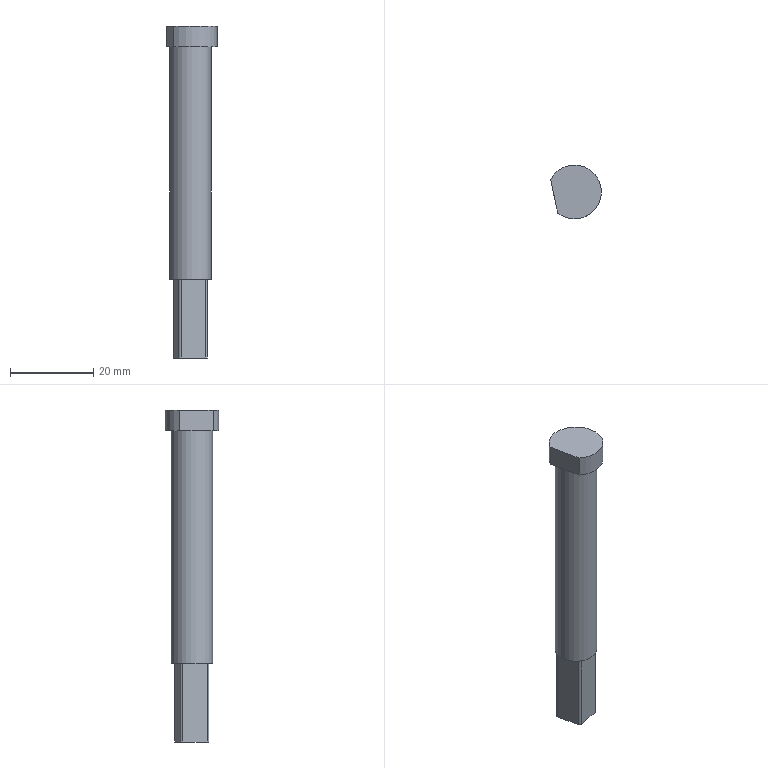Part | NX | features solid 2 | 1 solid | 15 faces | box 12.25 x 13 x 80 mm | volume 5972 mm3 | plane 9 | cylinder 6 | commonest cylinder face diameters 1.1 x4 10 x1 13 x1
STEP:
#1=CARTESIAN_POINT('',(-405.629,204.071,48.));
#2=VERTEX_POINT('',#1);
#3=CARTESIAN_POINT('',(-410.521,203.038,48.));
#4=DIRECTION('',(0.,0.,1.));
#5=DIRECTION('',(0.9784,0.2067,0.));
#6=AXIS2_PLACEMENT_3D('',#3,#4,#5);
#7=CIRCLE('',#6,5.);
#8=EDGE_CURVE('',#2,#2,#7,.T.);
#9=ORIENTED_EDGE('',*,*,#8,.F.);
#10=EDGE_LOOP('',(#9));
#11=FACE_BOUND('',#10,.T.);
#12=CARTESIAN_POINT('',(-414.615,205.239,48.));
#13=VERTEX_POINT('',#12);
#14=CARTESIAN_POINT('',(-413.375,199.369,48.));
#15=VERTEX_POINT('',#14);
#16=CARTESIAN_POINT('',(-414.728,205.778,48.));
#17=DIRECTION('',(0.2067,-0.9784,0.));
#18=VECTOR('',#17,1000.);
#19=LINE('',#16,#18);
#20=EDGE_CURVE('',#13,#15,#19,.T.);
#21=ORIENTED_EDGE('',*,*,#20,.T.);
#22=CARTESIAN_POINT('',(-412.723,198.944,48.));
#23=VERTEX_POINT('',#22);
#24=CARTESIAN_POINT('',(-412.837,199.483,48.));
#25=DIRECTION('',(0.,0.,1.));
#26=DIRECTION('',(0.9784,0.2067,0.));
#27=AXIS2_PLACEMENT_3D('',#24,#25,#26);
#28=CIRCLE('',#27,0.55);
#29=EDGE_CURVE('',#15,#23,#28,.T.);
#30=ORIENTED_EDGE('',*,*,#29,.T.);
#31=CARTESIAN_POINT('',(-406.852,200.184,48.));
#32=VERTEX_POINT('',#31);
#33=CARTESIAN_POINT('',(-413.261,198.831,48.));
#34=DIRECTION('',(0.9784,0.2067,0.));
#35=VECTOR('',#34,1000.);
#36=LINE('',#33,#35);
#37=EDGE_CURVE('',#23,#32,#36,.T.);
#38=ORIENTED_EDGE('',*,*,#37,.T.);
#39=CARTESIAN_POINT('',(-406.428,200.836,48.));
#40=VERTEX_POINT('',#39);
#41=CARTESIAN_POINT('',(-406.966,200.723,48.));
#42=DIRECTION('',(0.,0.,1.));
#43=DIRECTION('',(0.9784,0.2067,0.));
#44=AXIS2_PLACEMENT_3D('',#41,#42,#43);
#45=CIRCLE('',#44,0.55);
#46=EDGE_CURVE('',#32,#40,#45,.T.);
#47=ORIENTED_EDGE('',*,*,#46,.T.);
#48=CARTESIAN_POINT('',(-407.668,206.707,48.));
#49=VERTEX_POINT('',#48);
#50=CARTESIAN_POINT('',(-407.782,207.245,48.));
#51=DIRECTION('',(0.2067,-0.9784,0.));
#52=VECTOR('',#51,1000.);
#53=LINE('',#50,#52);
#54=EDGE_CURVE('',#49,#40,#53,.T.);
#55=ORIENTED_EDGE('',*,*,#54,.F.);
#56=CARTESIAN_POINT('',(-408.32,207.131,48.));
#57=VERTEX_POINT('',#56);
#58=CARTESIAN_POINT('',(-408.206,206.593,48.));
#59=DIRECTION('',(0.,0.,1.));
#60=DIRECTION('',(0.9784,0.2067,0.));
#61=AXIS2_PLACEMENT_3D('',#58,#59,#60);
#62=CIRCLE('',#61,0.55);
#63=EDGE_CURVE('',#49,#57,#62,.T.);
#64=ORIENTED_EDGE('',*,*,#63,.T.);
#65=CARTESIAN_POINT('',(-414.19,205.891,48.));
#66=VERTEX_POINT('',#65);
#67=CARTESIAN_POINT('',(-407.782,207.245,48.));
#68=DIRECTION('',(-0.9784,-0.2067,0.));
#69=VECTOR('',#68,1000.);
#70=LINE('',#67,#69);
#71=EDGE_CURVE('',#57,#66,#70,.T.);
#72=ORIENTED_EDGE('',*,*,#71,.T.);
#73=CARTESIAN_POINT('',(-414.076,205.353,48.));
#74=DIRECTION('',(0.,0.,1.));
#75=DIRECTION('',(0.9784,0.2067,0.));
#76=AXIS2_PLACEMENT_3D('',#73,#74,#75);
#77=CIRCLE('',#76,0.55);
#78=EDGE_CURVE('',#66,#13,#77,.T.);
#79=ORIENTED_EDGE('',*,*,#78,.T.);
#80=EDGE_LOOP('',(#21,#30,#38,#47,#55,#64,#72,#79));
#81=FACE_BOUND('',#80,.T.);
#82=CARTESIAN_POINT('',(-410.521,203.038,48.));
#83=DIRECTION('',(0.,0.,1.));
#84=DIRECTION('',(0.9784,0.2067,0.));
#85=AXIS2_PLACEMENT_3D('',#82,#83,#84);
#86=PLANE('',#85);
#87=ADVANCED_FACE('',(#11,#81),#86,.F.);
#88=ORIENTED_EDGE('',*,*,#8,.T.);
#89=EDGE_LOOP('',(#88));
#90=FACE_BOUND('',#89,.T.);
#91=CARTESIAN_POINT('',(-415.413,202.004,104.));
#92=VERTEX_POINT('',#91);
#93=CARTESIAN_POINT('',(-410.521,203.038,104.));
#94=DIRECTION('',(0.,0.,1.));
#95=DIRECTION('',(0.9784,0.2067,0.));
#96=AXIS2_PLACEMENT_3D('',#93,#94,#95);
#97=CIRCLE('',#96,5.);
#98=EDGE_CURVE('',#92,#92,#97,.T.);
#99=ORIENTED_EDGE('',*,*,#98,.F.);
#100=EDGE_LOOP('',(#99));
#101=FACE_BOUND('',#100,.T.);
#102=CARTESIAN_POINT('',(-410.521,203.038,109.));
#103=DIRECTION('',(0.,0.,-1.));
#104=DIRECTION('',(-0.9784,-0.2067,0.));
#105=AXIS2_PLACEMENT_3D('',#102,#103,#104);
#106=CYLINDRICAL_SURFACE('',#105,5.);
#107=ADVANCED_FACE('',(#90,#101),#106,.T.);
#108=CARTESIAN_POINT('',(-414.555,197.941,104.));
#109=VERTEX_POINT('',#108);
#110=CARTESIAN_POINT('',(-416.272,206.068,104.));
#111=VERTEX_POINT('',#110);
#112=CARTESIAN_POINT('',(-410.521,203.038,104.));
#113=DIRECTION('',(0.,0.,1.));
#114=DIRECTION('',(0.9784,0.2067,0.));
#115=AXIS2_PLACEMENT_3D('',#112,#113,#114);
#116=CIRCLE('',#115,6.5);
#117=EDGE_CURVE('',#109,#111,#116,.T.);
#118=ORIENTED_EDGE('',*,*,#117,.F.);
#119=CARTESIAN_POINT('',(-415.413,202.004,104.));
#120=DIRECTION('',(-0.2067,0.9784,0.));
#121=VECTOR('',#120,1000.);
#122=LINE('',#119,#121);
#123=EDGE_CURVE('',#109,#92,#122,.T.);
#124=ORIENTED_EDGE('',*,*,#123,.T.);
#125=ORIENTED_EDGE('',*,*,#98,.T.);
#126=CARTESIAN_POINT('',(-415.413,202.004,104.));
#127=DIRECTION('',(-0.2067,0.9784,0.));
#128=VECTOR('',#127,1000.);
#129=LINE('',#126,#128);
#130=EDGE_CURVE('',#92,#111,#129,.T.);
#131=ORIENTED_EDGE('',*,*,#130,.T.);
#132=EDGE_LOOP('',(#118,#124,#125,#131));
#133=FACE_BOUND('',#132,.T.);
#134=CARTESIAN_POINT('',(-410.521,203.038,104.));
#135=DIRECTION('',(0.,0.,1.));
#136=DIRECTION('',(0.9784,0.2067,0.));
#137=AXIS2_PLACEMENT_3D('',#134,#135,#136);
#138=PLANE('',#137);
#139=ADVANCED_FACE('',(#133),#138,.F.);
#140=CARTESIAN_POINT('',(-416.272,206.068,109.));
#141=VERTEX_POINT('',#140);
#142=CARTESIAN_POINT('',(-416.272,206.068,113.));
#143=DIRECTION('',(0.,0.,-1.));
#144=VECTOR('',#143,1000.);
#145=LINE('',#142,#144);
#146=EDGE_CURVE('',#141,#111,#145,.T.);
#147=ORIENTED_EDGE('',*,*,#146,.F.);
#148=CARTESIAN_POINT('',(-414.555,197.941,109.));
#149=VERTEX_POINT('',#148);
#150=CARTESIAN_POINT('',(-410.521,203.038,109.));
#151=DIRECTION('',(0.,0.,1.));
#152=DIRECTION('',(0.9784,0.2067,0.));
#153=AXIS2_PLACEMENT_3D('',#150,#151,#152);
#154=CIRCLE('',#153,6.5);
#155=EDGE_CURVE('',#149,#141,#154,.T.);
#156=ORIENTED_EDGE('',*,*,#155,.F.);
#157=CARTESIAN_POINT('',(-414.555,197.941,113.));
#158=DIRECTION('',(0.,0.,-1.));
#159=VECTOR('',#158,1000.);
#160=LINE('',#157,#159);
#161=EDGE_CURVE('',#109,#149,#160,.F.);
#162=ORIENTED_EDGE('',*,*,#161,.F.);
#163=ORIENTED_EDGE('',*,*,#117,.T.);
#164=EDGE_LOOP('',(#147,#156,#162,#163));
#165=FACE_BOUND('',#164,.T.);
#166=CARTESIAN_POINT('',(-410.521,203.038,104.));
#167=DIRECTION('',(0.,0.,1.));
#168=DIRECTION('',(0.9784,0.2067,0.));
#169=AXIS2_PLACEMENT_3D('',#166,#167,#168);
#170=CYLINDRICAL_SURFACE('',#169,6.5);
#171=ADVANCED_FACE('',(#165),#170,.T.);
#172=CARTESIAN_POINT('',(-415.413,202.004,109.));
#173=DIRECTION('',(-0.2067,0.9784,0.));
#174=VECTOR('',#173,1000.);
#175=LINE('',#172,#174);
#176=EDGE_CURVE('',#149,#141,#175,.T.);
#177=ORIENTED_EDGE('',*,*,#176,.F.);
#178=ORIENTED_EDGE('',*,*,#155,.T.);
#179=EDGE_LOOP('',(#177,#178));
#180=FACE_BOUND('',#179,.T.);
#181=CARTESIAN_POINT('',(-410.521,203.038,109.));
#182=DIRECTION('',(0.,0.,1.));
#183=DIRECTION('',(0.9784,0.2067,0.));
#184=AXIS2_PLACEMENT_3D('',#181,#182,#183);
#185=PLANE('',#184);
#186=ADVANCED_FACE('',(#180),#185,.T.);
#187=ORIENTED_EDGE('',*,*,#161,.T.);
#188=ORIENTED_EDGE('',*,*,#176,.T.);
#189=ORIENTED_EDGE('',*,*,#146,.T.);
#190=ORIENTED_EDGE('',*,*,#130,.F.);
#191=ORIENTED_EDGE('',*,*,#123,.F.);
#192=EDGE_LOOP('',(#187,#188,#189,#190,#191));
#193=FACE_BOUND('',#192,.T.);
#194=CARTESIAN_POINT('',(-416.272,206.068,113.));
#195=DIRECTION('',(0.9784,0.2067,0.));
#196=DIRECTION('',(0.,0.,-1.));
#197=AXIS2_PLACEMENT_3D('',#194,#195,#196);
#198=PLANE('',#197);
#199=ADVANCED_FACE('',(#193),#198,.F.);
#200=CARTESIAN_POINT('',(-412.723,198.944,29.));
#201=VERTEX_POINT('',#200);
#202=CARTESIAN_POINT('',(-406.852,200.184,29.));
#203=VERTEX_POINT('',#202);
#204=CARTESIAN_POINT('',(-413.261,198.831,29.));
#205=DIRECTION('',(0.9784,0.2067,0.));
#206=VECTOR('',#205,1000.);
#207=LINE('',#204,#206);
#208=EDGE_CURVE('',#201,#203,#207,.T.);
#209=ORIENTED_EDGE('',*,*,#208,.T.);
#210=CARTESIAN_POINT('',(-406.852,200.184,48.));
#211=DIRECTION('',(0.,0.,1.));
#212=VECTOR('',#211,1000.);
#213=LINE('',#210,#212);
#214=EDGE_CURVE('',#203,#32,#213,.T.);
#215=ORIENTED_EDGE('',*,*,#214,.T.);
#216=ORIENTED_EDGE('',*,*,#37,.F.);
#217=CARTESIAN_POINT('',(-412.723,198.944,29.));
#218=DIRECTION('',(0.,0.,1.));
#219=VECTOR('',#218,1000.);
#220=LINE('',#217,#219);
#221=EDGE_CURVE('',#23,#201,#220,.F.);
#222=ORIENTED_EDGE('',*,*,#221,.T.);
#223=EDGE_LOOP('',(#209,#215,#216,#222));
#224=FACE_BOUND('',#223,.T.);
#225=CARTESIAN_POINT('',(-413.261,198.831,29.));
#226=DIRECTION('',(0.2067,-0.9784,0.));
#227=DIRECTION('',(0.,0.,-1.));
#228=AXIS2_PLACEMENT_3D('',#225,#226,#227);
#229=PLANE('',#228);
#230=ADVANCED_FACE('',(#224),#229,.T.);
#231=CARTESIAN_POINT('',(-407.668,206.707,29.));
#232=VERTEX_POINT('',#231);
#233=CARTESIAN_POINT('',(-406.428,200.836,29.));
#234=VERTEX_POINT('',#233);
#235=CARTESIAN_POINT('',(-407.782,207.245,29.));
#236=DIRECTION('',(0.2067,-0.9784,0.));
#237=VECTOR('',#236,1000.);
#238=LINE('',#235,#237);
#239=EDGE_CURVE('',#232,#234,#238,.T.);
#240=ORIENTED_EDGE('',*,*,#239,.F.);
#241=CARTESIAN_POINT('',(-407.668,206.707,48.));
#242=DIRECTION('',(0.,0.,1.));
#243=VECTOR('',#242,1000.);
#244=LINE('',#241,#243);
#245=EDGE_CURVE('',#232,#49,#244,.T.);
#246=ORIENTED_EDGE('',*,*,#245,.T.);
#247=ORIENTED_EDGE('',*,*,#54,.T.);
#248=CARTESIAN_POINT('',(-406.428,200.836,29.));
#249=DIRECTION('',(0.,0.,1.));
#250=VECTOR('',#249,1000.);
#251=LINE('',#248,#250);
#252=EDGE_CURVE('',#40,#234,#251,.F.);
#253=ORIENTED_EDGE('',*,*,#252,.T.);
#254=EDGE_LOOP('',(#240,#246,#247,#253));
#255=FACE_BOUND('',#254,.T.);
#256=CARTESIAN_POINT('',(-407.782,207.245,29.));
#257=DIRECTION('',(-0.9784,-0.2067,0.));
#258=DIRECTION('',(0.,0.,1.));
#259=AXIS2_PLACEMENT_3D('',#256,#257,#258);
#260=PLANE('',#259);
#261=ADVANCED_FACE('',(#255),#260,.F.);
#262=ORIENTED_EDGE('',*,*,#71,.F.);
#263=CARTESIAN_POINT('',(-408.32,207.131,29.));
#264=VERTEX_POINT('',#263);
#265=CARTESIAN_POINT('',(-408.32,207.131,29.));
#266=DIRECTION('',(0.,0.,1.));
#267=VECTOR('',#266,1000.);
#268=LINE('',#265,#267);
#269=EDGE_CURVE('',#57,#264,#268,.F.);
#270=ORIENTED_EDGE('',*,*,#269,.T.);
#271=CARTESIAN_POINT('',(-414.19,205.891,29.));
#272=VERTEX_POINT('',#271);
#273=CARTESIAN_POINT('',(-407.782,207.245,29.));
#274=DIRECTION('',(-0.9784,-0.2067,0.));
#275=VECTOR('',#274,1000.);
#276=LINE('',#273,#275);
#277=EDGE_CURVE('',#264,#272,#276,.T.);
#278=ORIENTED_EDGE('',*,*,#277,.T.);
#279=CARTESIAN_POINT('',(-414.19,205.891,29.));
#280=DIRECTION('',(0.,0.,1.));
#281=VECTOR('',#280,1000.);
#282=LINE('',#279,#281);
#283=EDGE_CURVE('',#272,#66,#282,.T.);
#284=ORIENTED_EDGE('',*,*,#283,.T.);
#285=EDGE_LOOP('',(#262,#270,#278,#284));
#286=FACE_BOUND('',#285,.T.);
#287=CARTESIAN_POINT('',(-407.782,207.245,29.));
#288=DIRECTION('',(-0.2067,0.9784,0.));
#289=DIRECTION('',(0.,0.,1.));
#290=AXIS2_PLACEMENT_3D('',#287,#288,#289);
#291=PLANE('',#290);
#292=ADVANCED_FACE('',(#286),#291,.T.);
#293=ORIENTED_EDGE('',*,*,#20,.F.);
#294=CARTESIAN_POINT('',(-414.615,205.239,29.));
#295=VERTEX_POINT('',#294);
#296=CARTESIAN_POINT('',(-414.615,205.239,29.));
#297=DIRECTION('',(0.,0.,1.));
#298=VECTOR('',#297,1000.);
#299=LINE('',#296,#298);
#300=EDGE_CURVE('',#13,#295,#299,.F.);
#301=ORIENTED_EDGE('',*,*,#300,.T.);
#302=CARTESIAN_POINT('',(-413.375,199.369,29.));
#303=VERTEX_POINT('',#302);
#304=CARTESIAN_POINT('',(-414.728,205.778,29.));
#305=DIRECTION('',(0.2067,-0.9784,0.));
#306=VECTOR('',#305,1000.);
#307=LINE('',#304,#306);
#308=EDGE_CURVE('',#295,#303,#307,.T.);
#309=ORIENTED_EDGE('',*,*,#308,.T.);
#310=CARTESIAN_POINT('',(-413.375,199.369,29.));
#311=DIRECTION('',(0.,0.,1.));
#312=VECTOR('',#311,1000.);
#313=LINE('',#310,#312);
#314=EDGE_CURVE('',#303,#15,#313,.T.);
#315=ORIENTED_EDGE('',*,*,#314,.T.);
#316=EDGE_LOOP('',(#293,#301,#309,#315));
#317=FACE_BOUND('',#316,.T.);
#318=CARTESIAN_POINT('',(-414.728,205.778,29.));
#319=DIRECTION('',(-0.9784,-0.2067,0.));
#320=DIRECTION('',(0.,0.,1.));
#321=AXIS2_PLACEMENT_3D('',#318,#319,#320);
#322=PLANE('',#321);
#323=ADVANCED_FACE('',(#317),#322,.T.);
#324=ORIENTED_EDGE('',*,*,#277,.F.);
#325=CARTESIAN_POINT('',(-408.206,206.593,29.));
#326=DIRECTION('',(0.,0.,-1.));
#327=DIRECTION('',(-0.9784,-0.2067,0.));
#328=AXIS2_PLACEMENT_3D('',#325,#326,#327);
#329=CIRCLE('',#328,0.55);
#330=EDGE_CURVE('',#264,#232,#329,.T.);
#331=ORIENTED_EDGE('',*,*,#330,.T.);
#332=ORIENTED_EDGE('',*,*,#239,.T.);
#333=CARTESIAN_POINT('',(-406.966,200.723,29.));
#334=DIRECTION('',(0.,0.,-1.));
#335=DIRECTION('',(-0.9784,-0.2067,0.));
#336=AXIS2_PLACEMENT_3D('',#333,#334,#335);
#337=CIRCLE('',#336,0.55);
#338=EDGE_CURVE('',#234,#203,#337,.T.);
#339=ORIENTED_EDGE('',*,*,#338,.T.);
#340=ORIENTED_EDGE('',*,*,#208,.F.);
#341=CARTESIAN_POINT('',(-412.837,199.483,29.));
#342=DIRECTION('',(0.,0.,-1.));
#343=DIRECTION('',(-0.9784,-0.2067,0.));
#344=AXIS2_PLACEMENT_3D('',#341,#342,#343);
#345=CIRCLE('',#344,0.55);
#346=EDGE_CURVE('',#201,#303,#345,.T.);
#347=ORIENTED_EDGE('',*,*,#346,.T.);
#348=ORIENTED_EDGE('',*,*,#308,.F.);
#349=CARTESIAN_POINT('',(-414.076,205.353,29.));
#350=DIRECTION('',(0.,0.,-1.));
#351=DIRECTION('',(-0.9784,-0.2067,0.));
#352=AXIS2_PLACEMENT_3D('',#349,#350,#351);
#353=CIRCLE('',#352,0.55);
#354=EDGE_CURVE('',#295,#272,#353,.T.);
#355=ORIENTED_EDGE('',*,*,#354,.T.);
#356=EDGE_LOOP('',(#324,#331,#332,#339,#340,#347,#348,#355));
#357=FACE_BOUND('',#356,.T.);
#358=CARTESIAN_POINT('',(-406.314,200.298,29.));
#359=DIRECTION('',(0.,0.,-1.));
#360=DIRECTION('',(-0.9784,-0.2067,0.));
#361=AXIS2_PLACEMENT_3D('',#358,#359,#360);
#362=PLANE('',#361);
#363=ADVANCED_FACE('',(#357),#362,.T.);
#364=ORIENTED_EDGE('',*,*,#330,.F.);
#365=ORIENTED_EDGE('',*,*,#269,.F.);
#366=ORIENTED_EDGE('',*,*,#63,.F.);
#367=ORIENTED_EDGE('',*,*,#245,.F.);
#368=EDGE_LOOP('',(#364,#365,#366,#367));
#369=FACE_BOUND('',#368,.T.);
#370=CARTESIAN_POINT('',(-408.206,206.593,29.));
#371=DIRECTION('',(0.,0.,-1.));
#372=DIRECTION('',(-0.9784,-0.2067,0.));
#373=AXIS2_PLACEMENT_3D('',#370,#371,#372);
#374=CYLINDRICAL_SURFACE('',#373,0.55);
#375=ADVANCED_FACE('',(#369),#374,.T.);
#376=ORIENTED_EDGE('',*,*,#354,.F.);
#377=ORIENTED_EDGE('',*,*,#300,.F.);
#378=ORIENTED_EDGE('',*,*,#78,.F.);
#379=ORIENTED_EDGE('',*,*,#283,.F.);
#380=EDGE_LOOP('',(#376,#377,#378,#379));
#381=FACE_BOUND('',#380,.T.);
#382=CARTESIAN_POINT('',(-414.076,205.353,29.));
#383=DIRECTION('',(0.,0.,1.));
#384=DIRECTION('',(0.9784,0.2067,0.));
#385=AXIS2_PLACEMENT_3D('',#382,#383,#384);
#386=CYLINDRICAL_SURFACE('',#385,0.55);
#387=ADVANCED_FACE('',(#381),#386,.T.);
#388=ORIENTED_EDGE('',*,*,#338,.F.);
#389=ORIENTED_EDGE('',*,*,#252,.F.);
#390=ORIENTED_EDGE('',*,*,#46,.F.);
#391=ORIENTED_EDGE('',*,*,#214,.F.);
#392=EDGE_LOOP('',(#388,#389,#390,#391));
#393=FACE_BOUND('',#392,.T.);
#394=CARTESIAN_POINT('',(-406.966,200.723,29.));
#395=DIRECTION('',(0.,0.,-1.));
#396=DIRECTION('',(-0.9784,-0.2067,0.));
#397=AXIS2_PLACEMENT_3D('',#394,#395,#396);
#398=CYLINDRICAL_SURFACE('',#397,0.55);
#399=ADVANCED_FACE('',(#393),#398,.T.);
#400=ORIENTED_EDGE('',*,*,#346,.F.);
#401=ORIENTED_EDGE('',*,*,#221,.F.);
#402=ORIENTED_EDGE('',*,*,#29,.F.);
#403=ORIENTED_EDGE('',*,*,#314,.F.);
#404=EDGE_LOOP('',(#400,#401,#402,#403));
#405=FACE_BOUND('',#404,.T.);
#406=CARTESIAN_POINT('',(-412.837,199.483,29.));
#407=DIRECTION('',(0.,0.,1.));
#408=DIRECTION('',(0.9784,0.2067,0.));
#409=AXIS2_PLACEMENT_3D('',#406,#407,#408);
#410=CYLINDRICAL_SURFACE('',#409,0.55);
#411=ADVANCED_FACE('',(#405),#410,.T.);
#412=CLOSED_SHELL('',(#87,#107,#139,#171,#186,#199,#230,#261,#292,#323,#363,#375,#387,#399,#411));
#413=MANIFOLD_SOLID_BREP('',#412);
#414=(LENGTH_UNIT()NAMED_UNIT(*)SI_UNIT(.MILLI.,.METRE.));
#415=UNCERTAINTY_MEASURE_WITH_UNIT(LENGTH_MEASURE(0.00001),#414,'','');
#416=(NAMED_UNIT(*)PLANE_ANGLE_UNIT()SI_UNIT($,.RADIAN.));
#417=(NAMED_UNIT(*)SI_UNIT($,.STERADIAN.)SOLID_ANGLE_UNIT());
#418=(GEOMETRIC_REPRESENTATION_CONTEXT(3)GLOBAL_UNCERTAINTY_ASSIGNED_CONTEXT((#415))GLOBAL_UNIT_ASSIGNED_CONTEXT((#414,#416,#417))REPRESENTATION_CONTEXT('',''));
#419=ADVANCED_BREP_SHAPE_REPRESENTATION('',(#413),#418);